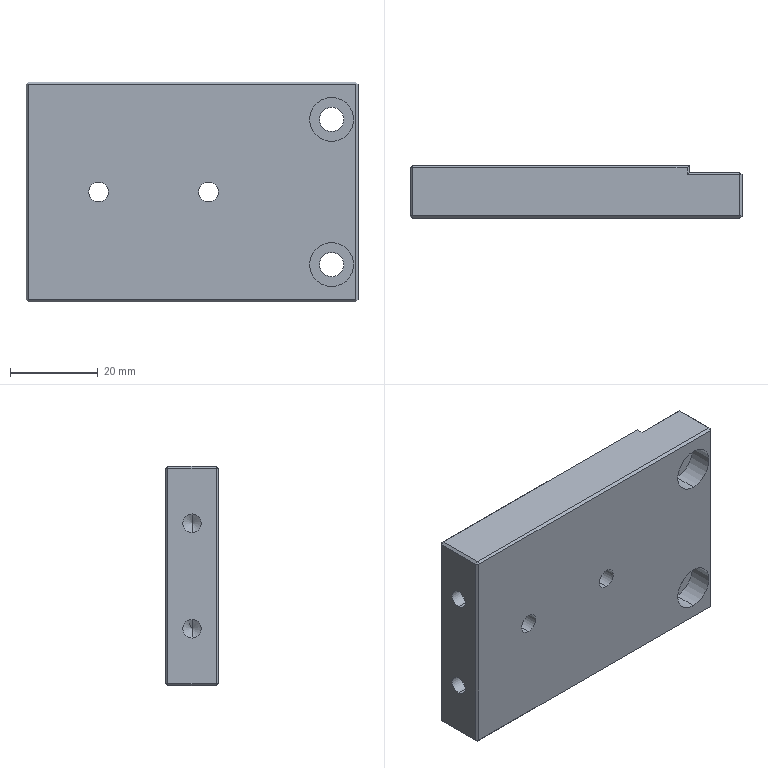Part | STEP file | ND25021-01-JDKM-25-TL | 1 solid | 60 faces | box 75.5 x 12 x 50 mm | volume 42202 mm3 | plane 36 | cylinder 20 | cone 4 | commonest cylinder face diameters 4.2 x4 4.5 x4 5.5 x4 8 x4 10 x4